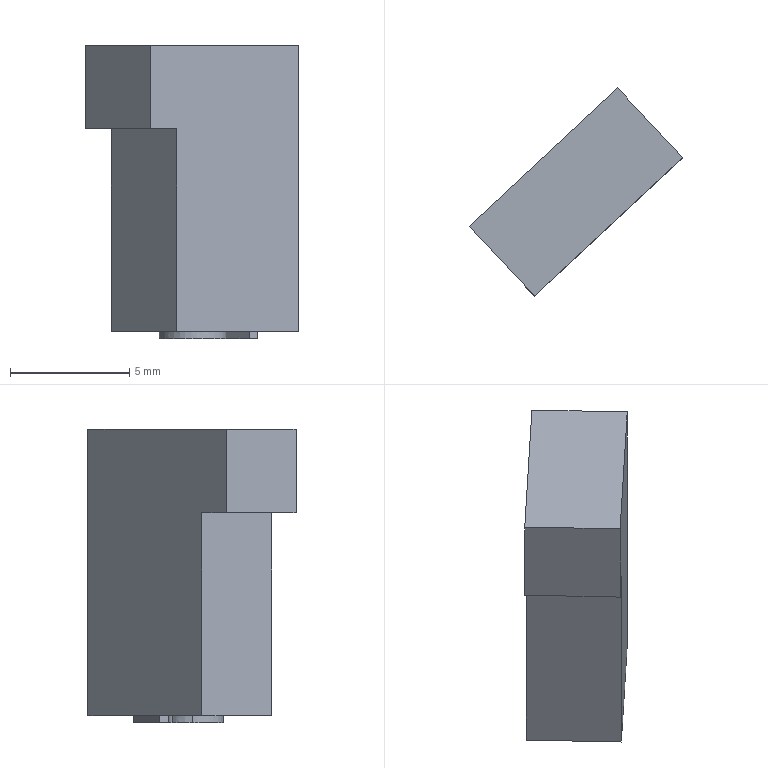Part | STEP file | gslz 2016.10.28-13_id954_x_t | 1 solid | 19 faces | box 8.945 x 8.722 x 12.3 mm | volume 358.338 mm3 | plane 16 | other 3